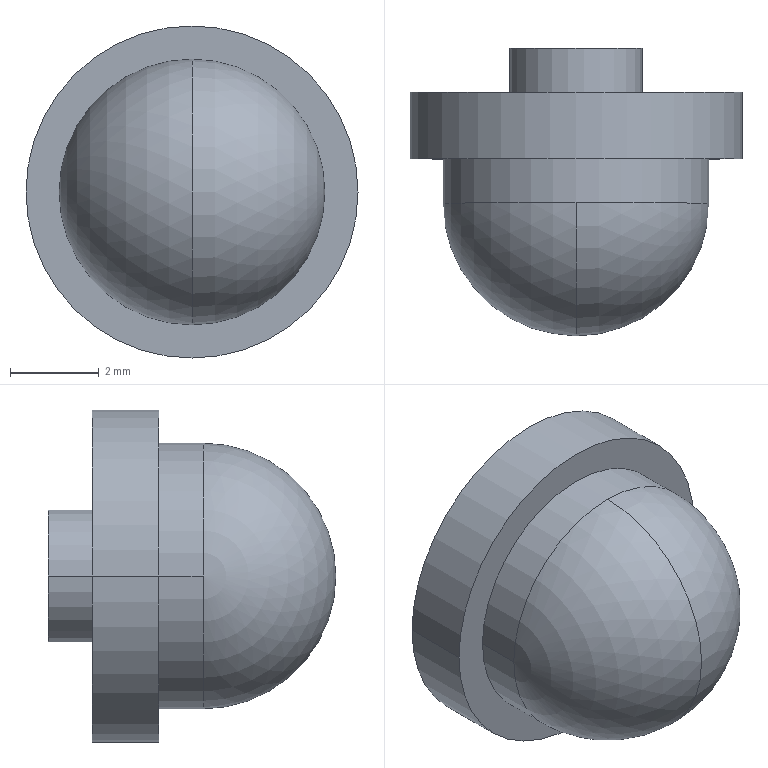Part | STEP file | SHS15C block-Part-2-7 | 1 solid | 11 faces | box 7.5 x 6.5 x 7.5 mm | volume 158.16 mm3 | cylinder 6 | plane 3 | sphere 2 | commonest cylinder face diameters 3 x2 6 x2 7.5 x2
STEP:
#1=CARTESIAN_POINT('',(0.,0.,0.));
#2=DIRECTION('',(0.,0.,1.));
#3=DIRECTION('',(1.,0.,0.));
#4=AXIS2_PLACEMENT_3D('',#1,#2,#3);
#5=CARTESIAN_POINT('',(61.7,-39.2,4.));
#6=VERTEX_POINT('',#5);
#7=CARTESIAN_POINT('',(58.7,-39.2,4.));
#8=VERTEX_POINT('',#7);
#9=CARTESIAN_POINT('',(60.2,-39.2,4.));
#10=DIRECTION('',(0.,-1.,0.));
#11=DIRECTION('',(-1.,0.,0.));
#12=AXIS2_PLACEMENT_3D('',#9,#10,#11);
#13=CIRCLE('',#12,1.5);
#14=CARTESIAN_POINT('',(60.2,-39.2,4.));
#15=DIRECTION('',(0.,-1.,0.));
#16=DIRECTION('',(1.,0.,0.));
#17=AXIS2_PLACEMENT_3D('',#14,#15,#16);
#18=CYLINDRICAL_SURFACE('',#17,1.5);
#19=CARTESIAN_POINT('',(-3.142,0.));
#20=DIRECTION('',(1.,0.));
#21=VECTOR('',#20,1.);
#22=LINE('',#19,#21);
#23=(GEOMETRIC_REPRESENTATION_CONTEXT(2)PARAMETRIC_REPRESENTATION_CONTEXT()REPRESENTATION_CONTEXT('',''));
#24=DEFINITIONAL_REPRESENTATION('',(#22),#23);
#25=PCURVE('',#18,#24);
#26=CARTESIAN_POINT('',(60.2,-39.2,4.));
#27=DIRECTION('',(0.,1.,0.));
#28=DIRECTION('',(-1.,0.,0.));
#29=AXIS2_PLACEMENT_3D('',#26,#27,#28);
#30=PLANE('',#29);
#31=CARTESIAN_POINT('',(1.5,0.));
#32=CARTESIAN_POINT('',(1.5,-2.598));
#33=CARTESIAN_POINT('',(-0.75,-1.299));
#34=CARTESIAN_POINT('',(-3.,0.));
#35=CARTESIAN_POINT('',(-0.75,1.299));
#36=CARTESIAN_POINT('',(1.5,2.598));
#37=CARTESIAN_POINT('',(1.5,0.));
#38=(BOUNDED_CURVE()B_SPLINE_CURVE(2,(#31,#32,#33,#34,#35,#36,#37),.UNSPECIFIED.,.T.,.F.)B_SPLINE_CURVE_WITH_KNOTS((1,2,2,2,2,1),(-2.094,0.,2.094,4.189,6.283,8.378),.UNSPECIFIED.)CURVE()GEOMETRIC_REPRESENTATION_ITEM()RATIONAL_B_SPLINE_CURVE((1.,0.5,1.,0.5,1.,0.5,1.))REPRESENTATION_ITEM(''));
#39=(GEOMETRIC_REPRESENTATION_CONTEXT(2)PARAMETRIC_REPRESENTATION_CONTEXT()REPRESENTATION_CONTEXT('',''));
#40=DEFINITIONAL_REPRESENTATION('',(#38),#39);
#41=PCURVE('',#30,#40);
#42=SURFACE_CURVE('',#13,(#25,#41),.PCURVE_S1.);
#43=EDGE_CURVE('',#6,#8,#42,.T.);
#44=ORIENTED_EDGE('',*,*,#43,.T.);
#45=CARTESIAN_POINT('',(58.7,-40.2,4.));
#46=VERTEX_POINT('',#45);
#47=CARTESIAN_POINT('',(58.7,-39.2,4.));
#48=DIRECTION('',(0.,-1.,0.));
#49=VECTOR('',#48,1.);
#50=LINE('',#47,#49);
#51=CARTESIAN_POINT('',(3.142,0.));
#52=DIRECTION('',(0.,1.));
#53=VECTOR('',#52,1.);
#54=LINE('',#51,#53);
#55=(GEOMETRIC_REPRESENTATION_CONTEXT(2)PARAMETRIC_REPRESENTATION_CONTEXT()REPRESENTATION_CONTEXT('',''));
#56=DEFINITIONAL_REPRESENTATION('',(#54),#55);
#57=PCURVE('',#18,#56);
#58=CARTESIAN_POINT('',(60.2,-39.2,4.));
#59=DIRECTION('',(0.,-1.,0.));
#60=DIRECTION('',(1.,0.,0.));
#61=AXIS2_PLACEMENT_3D('',#58,#59,#60);
#62=CYLINDRICAL_SURFACE('',#61,1.5);
#63=CARTESIAN_POINT('',(3.142,0.));
#64=DIRECTION('',(0.,1.));
#65=VECTOR('',#64,1.);
#66=LINE('',#63,#65);
#67=(GEOMETRIC_REPRESENTATION_CONTEXT(2)PARAMETRIC_REPRESENTATION_CONTEXT()REPRESENTATION_CONTEXT('',''));
#68=DEFINITIONAL_REPRESENTATION('',(#66),#67);
#69=PCURVE('',#62,#68);
#70=SURFACE_CURVE('',#50,(#57,#69),.PCURVE_S1.);
#71=EDGE_CURVE('',#8,#46,#70,.T.);
#72=ORIENTED_EDGE('',*,*,#71,.T.);
#73=CARTESIAN_POINT('',(61.7,-40.2,4.));
#74=VERTEX_POINT('',#73);
#75=CARTESIAN_POINT('',(60.2,-40.2,4.));
#76=DIRECTION('',(0.,-1.,0.));
#77=DIRECTION('',(-1.,0.,0.));
#78=AXIS2_PLACEMENT_3D('',#75,#76,#77);
#79=CIRCLE('',#78,1.5);
#80=CARTESIAN_POINT('',(-3.142,1.));
#81=DIRECTION('',(1.,0.));
#82=VECTOR('',#81,1.);
#83=LINE('',#80,#82);
#84=(GEOMETRIC_REPRESENTATION_CONTEXT(2)PARAMETRIC_REPRESENTATION_CONTEXT()REPRESENTATION_CONTEXT('',''));
#85=DEFINITIONAL_REPRESENTATION('',(#83),#84);
#86=PCURVE('',#18,#85);
#87=CARTESIAN_POINT('',(60.2,-40.2,0.25));
#88=DIRECTION('',(0.,-1.,0.));
#89=DIRECTION('',(1.,0.,0.));
#90=AXIS2_PLACEMENT_3D('',#87,#88,#89);
#91=PLANE('',#90);
#92=CARTESIAN_POINT('',(0.,3.75));
#93=DIRECTION('',(-1.,0.));
#94=AXIS2_PLACEMENT_2D('',#92,#93);
#95=CIRCLE('',#94,1.5);
#96=(GEOMETRIC_REPRESENTATION_CONTEXT(2)PARAMETRIC_REPRESENTATION_CONTEXT()REPRESENTATION_CONTEXT('',''));
#97=DEFINITIONAL_REPRESENTATION('',(#95),#96);
#98=PCURVE('',#91,#97);
#99=SURFACE_CURVE('',#79,(#86,#98),.PCURVE_S1.);
#100=EDGE_CURVE('',#74,#46,#99,.T.);
#101=ORIENTED_EDGE('',*,*,#100,.F.);
#102=CARTESIAN_POINT('',(61.7,-39.2,4.));
#103=DIRECTION('',(0.,-1.,0.));
#104=VECTOR('',#103,1.);
#105=LINE('',#102,#104);
#106=CARTESIAN_POINT('',(0.,0.));
#107=DIRECTION('',(0.,1.));
#108=VECTOR('',#107,1.);
#109=LINE('',#106,#108);
#110=(GEOMETRIC_REPRESENTATION_CONTEXT(2)PARAMETRIC_REPRESENTATION_CONTEXT()REPRESENTATION_CONTEXT('',''));
#111=DEFINITIONAL_REPRESENTATION('',(#109),#110);
#112=PCURVE('',#18,#111);
#113=CARTESIAN_POINT('',(6.283,0.));
#114=DIRECTION('',(0.,1.));
#115=VECTOR('',#114,1.);
#116=LINE('',#113,#115);
#117=(GEOMETRIC_REPRESENTATION_CONTEXT(2)PARAMETRIC_REPRESENTATION_CONTEXT()REPRESENTATION_CONTEXT('',''));
#118=DEFINITIONAL_REPRESENTATION('',(#116),#117);
#119=PCURVE('',#62,#118);
#120=SURFACE_CURVE('',#105,(#112,#119),.PCURVE_S1.);
#121=EDGE_CURVE('',#6,#74,#120,.T.);
#122=ORIENTED_EDGE('',*,*,#121,.F.);
#123=EDGE_LOOP('',(#44,#72,#101,#122));
#124=FACE_BOUND('',#123,.T.);
#125=ADVANCED_FACE('',(#124),#18,.T.);
#126=CARTESIAN_POINT('',(63.95,-41.7,4.));
#127=VERTEX_POINT('',#126);
#128=CARTESIAN_POINT('',(56.45,-41.7,4.));
#129=VERTEX_POINT('',#128);
#130=CARTESIAN_POINT('',(60.2,-41.7,4.));
#131=DIRECTION('',(0.,-1.,0.));
#132=DIRECTION('',(-1.,0.,0.));
#133=AXIS2_PLACEMENT_3D('',#130,#131,#132);
#134=CIRCLE('',#133,3.75);
#135=CARTESIAN_POINT('',(60.2,-35.7,4.));
#136=DIRECTION('',(0.,1.,0.));
#137=DIRECTION('',(-1.,0.,0.));
#138=AXIS2_PLACEMENT_3D('',#135,#136,#137);
#139=CYLINDRICAL_SURFACE('',#138,3.75);
#140=CARTESIAN_POINT('',(6.283,-6.));
#141=DIRECTION('',(-1.,0.));
#142=VECTOR('',#141,1.);
#143=LINE('',#140,#142);
#144=(GEOMETRIC_REPRESENTATION_CONTEXT(2)PARAMETRIC_REPRESENTATION_CONTEXT()REPRESENTATION_CONTEXT('',''));
#145=DEFINITIONAL_REPRESENTATION('',(#143),#144);
#146=PCURVE('',#139,#145);
#147=CARTESIAN_POINT('',(60.2,-41.7,1.));
#148=DIRECTION('',(0.,1.,0.));
#149=DIRECTION('',(-1.,0.,0.));
#150=AXIS2_PLACEMENT_3D('',#147,#148,#149);
#151=PLANE('',#150);
#152=CARTESIAN_POINT('',(3.75,3.));
#153=CARTESIAN_POINT('',(3.75,-3.495));
#154=CARTESIAN_POINT('',(-1.875,-0.2476));
#155=CARTESIAN_POINT('',(-7.5,3.));
#156=CARTESIAN_POINT('',(-1.875,6.248));
#157=CARTESIAN_POINT('',(3.75,9.495));
#158=CARTESIAN_POINT('',(3.75,3.));
#159=(BOUNDED_CURVE()B_SPLINE_CURVE(2,(#152,#153,#154,#155,#156,#157,#158),.UNSPECIFIED.,.T.,.F.)B_SPLINE_CURVE_WITH_KNOTS((1,2,2,2,2,1),(-2.094,0.,2.094,4.189,6.283,8.378),.UNSPECIFIED.)CURVE()GEOMETRIC_REPRESENTATION_ITEM()RATIONAL_B_SPLINE_CURVE((1.,0.5,1.,0.5,1.,0.5,1.))REPRESENTATION_ITEM(''));
#160=(GEOMETRIC_REPRESENTATION_CONTEXT(2)PARAMETRIC_REPRESENTATION_CONTEXT()REPRESENTATION_CONTEXT('',''));
#161=DEFINITIONAL_REPRESENTATION('',(#159),#160);
#162=PCURVE('',#151,#161);
#163=SURFACE_CURVE('',#134,(#146,#162),.PCURVE_S1.);
#164=EDGE_CURVE('',#127,#129,#163,.T.);
#165=ORIENTED_EDGE('',*,*,#164,.F.);
#166=CARTESIAN_POINT('',(63.95,-40.2,4.));
#167=VERTEX_POINT('',#166);
#168=CARTESIAN_POINT('',(63.95,-35.7,4.));
#169=DIRECTION('',(0.,1.,0.));
#170=VECTOR('',#169,1.);
#171=LINE('',#168,#170);
#172=CARTESIAN_POINT('',(3.142,0.));
#173=DIRECTION('',(0.,1.));
#174=VECTOR('',#173,1.);
#175=LINE('',#172,#174);
#176=(GEOMETRIC_REPRESENTATION_CONTEXT(2)PARAMETRIC_REPRESENTATION_CONTEXT()REPRESENTATION_CONTEXT('',''));
#177=DEFINITIONAL_REPRESENTATION('',(#175),#176);
#178=PCURVE('',#139,#177);
#179=CARTESIAN_POINT('',(60.2,-35.7,4.));
#180=DIRECTION('',(0.,1.,0.));
#181=DIRECTION('',(-1.,0.,0.));
#182=AXIS2_PLACEMENT_3D('',#179,#180,#181);
#183=CYLINDRICAL_SURFACE('',#182,3.75);
#184=CARTESIAN_POINT('',(3.142,0.));
#185=DIRECTION('',(0.,1.));
#186=VECTOR('',#185,1.);
#187=LINE('',#184,#186);
#188=(GEOMETRIC_REPRESENTATION_CONTEXT(2)PARAMETRIC_REPRESENTATION_CONTEXT()REPRESENTATION_CONTEXT('',''));
#189=DEFINITIONAL_REPRESENTATION('',(#187),#188);
#190=PCURVE('',#183,#189);
#191=SURFACE_CURVE('',#171,(#178,#190),.PCURVE_S1.);
#192=EDGE_CURVE('',#127,#167,#191,.T.);
#193=ORIENTED_EDGE('',*,*,#192,.T.);
#194=CARTESIAN_POINT('',(56.45,-40.2,4.));
#195=VERTEX_POINT('',#194);
#196=CARTESIAN_POINT('',(60.2,-40.2,4.));
#197=DIRECTION('',(0.,-1.,0.));
#198=DIRECTION('',(-1.,0.,0.));
#199=AXIS2_PLACEMENT_3D('',#196,#197,#198);
#200=CIRCLE('',#199,3.75);
#201=CARTESIAN_POINT('',(6.283,-4.5));
#202=DIRECTION('',(-1.,0.));
#203=VECTOR('',#202,1.);
#204=LINE('',#201,#203);
#205=(GEOMETRIC_REPRESENTATION_CONTEXT(2)PARAMETRIC_REPRESENTATION_CONTEXT()REPRESENTATION_CONTEXT('',''));
#206=DEFINITIONAL_REPRESENTATION('',(#204),#205);
#207=PCURVE('',#139,#206);
#208=CARTESIAN_POINT('',(0.,3.75));
#209=DIRECTION('',(-1.,0.));
#210=AXIS2_PLACEMENT_2D('',#208,#209);
#211=CIRCLE('',#210,3.75);
#212=(GEOMETRIC_REPRESENTATION_CONTEXT(2)PARAMETRIC_REPRESENTATION_CONTEXT()REPRESENTATION_CONTEXT('',''));
#213=DEFINITIONAL_REPRESENTATION('',(#211),#212);
#214=PCURVE('',#91,#213);
#215=SURFACE_CURVE('',#200,(#207,#214),.PCURVE_S1.);
#216=EDGE_CURVE('',#167,#195,#215,.T.);
#217=ORIENTED_EDGE('',*,*,#216,.T.);
#218=CARTESIAN_POINT('',(56.45,-35.7,4.));
#219=DIRECTION('',(0.,1.,0.));
#220=VECTOR('',#219,1.);
#221=LINE('',#218,#220);
#222=CARTESIAN_POINT('',(0.,0.));
#223=DIRECTION('',(0.,1.));
#224=VECTOR('',#223,1.);
#225=LINE('',#222,#224);
#226=(GEOMETRIC_REPRESENTATION_CONTEXT(2)PARAMETRIC_REPRESENTATION_CONTEXT()REPRESENTATION_CONTEXT('',''));
#227=DEFINITIONAL_REPRESENTATION('',(#225),#226);
#228=PCURVE('',#139,#227);
#229=CARTESIAN_POINT('',(6.283,0.));
#230=DIRECTION('',(0.,1.));
#231=VECTOR('',#230,1.);
#232=LINE('',#229,#231);
#233=(GEOMETRIC_REPRESENTATION_CONTEXT(2)PARAMETRIC_REPRESENTATION_CONTEXT()REPRESENTATION_CONTEXT('',''));
#234=DEFINITIONAL_REPRESENTATION('',(#232),#233);
#235=PCURVE('',#183,#234);
#236=SURFACE_CURVE('',#221,(#228,#235),.PCURVE_S1.);
#237=EDGE_CURVE('',#129,#195,#236,.T.);
#238=ORIENTED_EDGE('',*,*,#237,.F.);
#239=EDGE_LOOP('',(#165,#193,#217,#238));
#240=FACE_BOUND('',#239,.T.);
#241=ADVANCED_FACE('',(#240),#139,.T.);
#242=CARTESIAN_POINT('',(63.2,-42.7,4.));
#243=VERTEX_POINT('',#242);
#244=CARTESIAN_POINT('',(60.2,-42.7,7.));
#245=VERTEX_POINT('',#244);
#246=CARTESIAN_POINT('',(60.2,-42.7,4.));
#247=DIRECTION('',(0.,-1.,0.));
#248=DIRECTION('',(-1.,0.,0.));
#249=AXIS2_PLACEMENT_3D('',#246,#247,#248);
#250=CIRCLE('',#249,3.);
#251=CARTESIAN_POINT('',(60.2,-35.7,4.));
#252=DIRECTION('',(0.,1.,0.));
#253=DIRECTION('',(-1.,0.,0.));
#254=AXIS2_PLACEMENT_3D('',#251,#252,#253);
#255=CYLINDRICAL_SURFACE('',#254,3.);
#256=CARTESIAN_POINT('',(6.283,-7.));
#257=DIRECTION('',(-1.,0.));
#258=VECTOR('',#257,1.);
#259=LINE('',#256,#258);
#260=(GEOMETRIC_REPRESENTATION_CONTEXT(2)PARAMETRIC_REPRESENTATION_CONTEXT()REPRESENTATION_CONTEXT('',''));
#261=DEFINITIONAL_REPRESENTATION('',(#259),#260);
#262=PCURVE('',#255,#261);
#263=CARTESIAN_POINT('',(60.2,-42.7,4.));
#264=DIRECTION('',(-1.,0.,0.));
#265=DIRECTION('',(0.,0.,-1.));
#266=AXIS2_PLACEMENT_3D('',#263,#264,#265);
#267=SPHERICAL_SURFACE('',#266,3.);
#268=CARTESIAN_POINT('',(3.142,-1.571));
#269=CARTESIAN_POINT('',(3.142,-1.547));
#270=CARTESIAN_POINT('',(3.142,-1.499));
#271=CARTESIAN_POINT('',(3.142,-1.428));
#272=CARTESIAN_POINT('',(3.142,-1.357));
#273=CARTESIAN_POINT('',(3.142,-1.285));
#274=CARTESIAN_POINT('',(3.142,-1.214));
#275=CARTESIAN_POINT('',(3.142,-1.142));
#276=CARTESIAN_POINT('',(3.142,-1.071));
#277=CARTESIAN_POINT('',(3.142,-0.9996));
#278=CARTESIAN_POINT('',(3.142,-0.9282));
#279=CARTESIAN_POINT('',(3.142,-0.8568));
#280=CARTESIAN_POINT('',(3.142,-0.7854));
#281=CARTESIAN_POINT('',(3.142,-0.714));
#282=CARTESIAN_POINT('',(3.142,-0.6426));
#283=CARTESIAN_POINT('',(3.142,-0.5712));
#284=CARTESIAN_POINT('',(3.142,-0.4998));
#285=CARTESIAN_POINT('',(3.142,-0.4284));
#286=CARTESIAN_POINT('',(3.142,-0.357));
#287=CARTESIAN_POINT('',(3.142,-0.2856));
#288=CARTESIAN_POINT('',(3.142,-0.2142));
#289=CARTESIAN_POINT('',(3.142,-0.1428));
#290=CARTESIAN_POINT('',(3.142,-0.0714));
#291=CARTESIAN_POINT('',(3.142,-0.0238));
#292=CARTESIAN_POINT('',(3.142,0.));
#293=B_SPLINE_CURVE_WITH_KNOTS('',3,(#268,#269,#270,#271,#272,#273,#274,#275,#276,#277,#278,#279,#280,#281,#282,#283,#284,#285,#286,#287,#288,#289,#290,#291,#292),.UNSPECIFIED.,.F.,.F.,(4,1,1,1,1,1,1,1,1,1,1,1,1,1,1,1,1,1,1,1,1,1,4),(3.142,3.213,3.284,3.356,3.427,3.499,3.57,3.641,3.713,3.784,3.856,3.927,3.998,4.07,4.141,4.213,4.284,4.355,4.427,4.498,4.57,4.641,4.712),.QUASI_UNIFORM_KNOTS.);
#294=(GEOMETRIC_REPRESENTATION_CONTEXT(2)PARAMETRIC_REPRESENTATION_CONTEXT()REPRESENTATION_CONTEXT('',''));
#295=DEFINITIONAL_REPRESENTATION('',(#293),#294);
#296=PCURVE('',#267,#295);
#297=SURFACE_CURVE('',#250,(#262,#296),.PCURVE_S1.);
#298=EDGE_CURVE('',#243,#245,#297,.T.);
#299=ORIENTED_EDGE('',*,*,#298,.F.);
#300=CARTESIAN_POINT('',(63.2,-41.7,4.));
#301=VERTEX_POINT('',#300);
#302=CARTESIAN_POINT('',(63.2,-35.7,4.));
#303=DIRECTION('',(0.,1.,0.));
#304=VECTOR('',#303,1.);
#305=LINE('',#302,#304);
#306=CARTESIAN_POINT('',(3.142,0.));
#307=DIRECTION('',(0.,1.));
#308=VECTOR('',#307,1.);
#309=LINE('',#306,#308);
#310=(GEOMETRIC_REPRESENTATION_CONTEXT(2)PARAMETRIC_REPRESENTATION_CONTEXT()REPRESENTATION_CONTEXT('',''));
#311=DEFINITIONAL_REPRESENTATION('',(#309),#310);
#312=PCURVE('',#255,#311);
#313=CARTESIAN_POINT('',(60.2,-35.7,4.));
#314=DIRECTION('',(0.,1.,0.));
#315=DIRECTION('',(-1.,0.,0.));
#316=AXIS2_PLACEMENT_3D('',#313,#314,#315);
#317=CYLINDRICAL_SURFACE('',#316,3.);
#318=CARTESIAN_POINT('',(3.142,0.));
#319=DIRECTION('',(0.,1.));
#320=VECTOR('',#319,1.);
#321=LINE('',#318,#320);
#322=(GEOMETRIC_REPRESENTATION_CONTEXT(2)PARAMETRIC_REPRESENTATION_CONTEXT()REPRESENTATION_CONTEXT('',''));
#323=DEFINITIONAL_REPRESENTATION('',(#321),#322);
#324=PCURVE('',#317,#323);
#325=SURFACE_CURVE('',#305,(#312,#324),.PCURVE_S1.);
#326=EDGE_CURVE('',#243,#301,#325,.T.);
#327=ORIENTED_EDGE('',*,*,#326,.T.);
#328=CARTESIAN_POINT('',(57.2,-41.7,4.));
#329=VERTEX_POINT('',#328);
#330=CARTESIAN_POINT('',(60.2,-41.7,4.));
#331=DIRECTION('',(0.,-1.,0.));
#332=DIRECTION('',(-1.,0.,0.));
#333=AXIS2_PLACEMENT_3D('',#330,#331,#332);
#334=CIRCLE('',#333,3.);
#335=CARTESIAN_POINT('',(6.283,-6.));
#336=DIRECTION('',(-1.,0.));
#337=VECTOR('',#336,1.);
#338=LINE('',#335,#337);
#339=(GEOMETRIC_REPRESENTATION_CONTEXT(2)PARAMETRIC_REPRESENTATION_CONTEXT()REPRESENTATION_CONTEXT('',''));
#340=DEFINITIONAL_REPRESENTATION('',(#338),#339);
#341=PCURVE('',#255,#340);
#342=CARTESIAN_POINT('',(3.,3.));
#343=CARTESIAN_POINT('',(3.,-2.196));
#344=CARTESIAN_POINT('',(-1.5,0.4019));
#345=CARTESIAN_POINT('',(-6.,3.));
#346=CARTESIAN_POINT('',(-1.5,5.598));
#347=CARTESIAN_POINT('',(3.,8.196));
#348=CARTESIAN_POINT('',(3.,3.));
#349=(BOUNDED_CURVE()B_SPLINE_CURVE(2,(#342,#343,#344,#345,#346,#347,#348),.UNSPECIFIED.,.T.,.F.)B_SPLINE_CURVE_WITH_KNOTS((1,2,2,2,2,1),(-2.094,0.,2.094,4.189,6.283,8.378),.UNSPECIFIED.)CURVE()GEOMETRIC_REPRESENTATION_ITEM()RATIONAL_B_SPLINE_CURVE((1.,0.5,1.,0.5,1.,0.5,1.))REPRESENTATION_ITEM(''));
#350=(GEOMETRIC_REPRESENTATION_CONTEXT(2)PARAMETRIC_REPRESENTATION_CONTEXT()REPRESENTATION_CONTEXT('',''));
#351=DEFINITIONAL_REPRESENTATION('',(#349),#350);
#352=PCURVE('',#151,#351);
#353=SURFACE_CURVE('',#334,(#341,#352),.PCURVE_S1.);
#354=EDGE_CURVE('',#301,#329,#353,.T.);
#355=ORIENTED_EDGE('',*,*,#354,.T.);
#356=CARTESIAN_POINT('',(57.2,-42.7,4.));
#357=VERTEX_POINT('',#356);
#358=CARTESIAN_POINT('',(57.2,-35.7,4.));
#359=DIRECTION('',(0.,1.,0.));
#360=VECTOR('',#359,1.);
#361=LINE('',#358,#360);
#362=CARTESIAN_POINT('',(0.,0.));
#363=DIRECTION('',(0.,1.));
#364=VECTOR('',#363,1.);
#365=LINE('',#362,#364);
#366=(GEOMETRIC_REPRESENTATION_CONTEXT(2)PARAMETRIC_REPRESENTATION_CONTEXT()REPRESENTATION_CONTEXT('',''));
#367=DEFINITIONAL_REPRESENTATION('',(#365),#366);
#368=PCURVE('',#255,#367);
#369=CARTESIAN_POINT('',(6.283,0.));
#370=DIRECTION('',(0.,1.));
#371=VECTOR('',#370,1.);
#372=LINE('',#369,#371);
#373=(GEOMETRIC_REPRESENTATION_CONTEXT(2)PARAMETRIC_REPRESENTATION_CONTEXT()REPRESENTATION_CONTEXT('',''));
#374=DEFINITIONAL_REPRESENTATION('',(#372),#373);
#375=PCURVE('',#317,#374);
#376=SURFACE_CURVE('',#361,(#368,#375),.PCURVE_S1.);
#377=EDGE_CURVE('',#357,#329,#376,.T.);
#378=ORIENTED_EDGE('',*,*,#377,.F.);
#379=CARTESIAN_POINT('',(60.2,-42.7,4.));
#380=DIRECTION('',(0.,-1.,0.));
#381=DIRECTION('',(-1.,0.,0.));
#382=AXIS2_PLACEMENT_3D('',#379,#380,#381);
#383=CIRCLE('',#382,3.);
#384=CARTESIAN_POINT('',(6.283,-7.));
#385=DIRECTION('',(-1.,0.));
#386=VECTOR('',#385,1.);
#387=LINE('',#384,#386);
#388=(GEOMETRIC_REPRESENTATION_CONTEXT(2)PARAMETRIC_REPRESENTATION_CONTEXT()REPRESENTATION_CONTEXT('',''));
#389=DEFINITIONAL_REPRESENTATION('',(#387),#388);
#390=PCURVE('',#255,#389);
#391=CARTESIAN_POINT('',(60.2,-42.7,4.));
#392=DIRECTION('',(-1.,0.,0.));
#393=DIRECTION('',(0.,0.,-1.));
#394=AXIS2_PLACEMENT_3D('',#391,#392,#393);
#395=SPHERICAL_SURFACE('',#394,3.);
#396=CARTESIAN_POINT('',(3.142,-4.712));
#397=DIRECTION('',(0.,1.));
#398=VECTOR('',#397,1.);
#399=LINE('',#396,#398);
#400=(GEOMETRIC_REPRESENTATION_CONTEXT(2)PARAMETRIC_REPRESENTATION_CONTEXT()REPRESENTATION_CONTEXT('',''));
#401=DEFINITIONAL_REPRESENTATION('',(#399),#400);
#402=PCURVE('',#395,#401);
#403=SURFACE_CURVE('',#383,(#390,#402),.PCURVE_S1.);
#404=EDGE_CURVE('',#245,#357,#403,.T.);
#405=ORIENTED_EDGE('',*,*,#404,.F.);
#406=EDGE_LOOP('',(#299,#327,#355,#378,#405));
#407=FACE_BOUND('',#406,.T.);
#408=ADVANCED_FACE('',(#407),#255,.T.);
#409=CARTESIAN_POINT('',(60.2,-45.7,4.));
#410=VERTEX_POINT('',#409);
#411=CARTESIAN_POINT('',(60.2,-42.7,1.));
#412=VERTEX_POINT('',#411);
#413=CARTESIAN_POINT('',(60.2,-42.7,4.));
#414=DIRECTION('',(1.,0.,0.));
#415=DIRECTION('',(0.,0.,-1.));
#416=AXIS2_PLACEMENT_3D('',#413,#414,#415);
#417=CIRCLE('',#416,3.);
#418=CARTESIAN_POINT('',(6.283,0.));
#419=DIRECTION('',(-1.,0.));
#420=VECTOR('',#419,1.);
#421=LINE('',#418,#420);
#422=(GEOMETRIC_REPRESENTATION_CONTEXT(2)PARAMETRIC_REPRESENTATION_CONTEXT()REPRESENTATION_CONTEXT('',''));
#423=DEFINITIONAL_REPRESENTATION('',(#421),#422);
#424=PCURVE('',#395,#423);
#425=CARTESIAN_POINT('',(6.283,0.));
#426=DIRECTION('',(-1.,0.));
#427=VECTOR('',#426,1.);
#428=LINE('',#425,#427);
#429=(GEOMETRIC_REPRESENTATION_CONTEXT(2)PARAMETRIC_REPRESENTATION_CONTEXT()REPRESENTATION_CONTEXT('',''));
#430=DEFINITIONAL_REPRESENTATION('',(#428),#429);
#431=PCURVE('',#267,#430);
#432=SURFACE_CURVE('',#417,(#424,#431),.PCURVE_S1.);
#433=EDGE_CURVE('',#410,#412,#432,.T.);
#434=ORIENTED_EDGE('',*,*,#433,.F.);
#435=CARTESIAN_POINT('',(60.2,-42.7,4.));
#436=DIRECTION('',(-1.,0.,0.));
#437=DIRECTION('',(0.,0.,1.));
#438=AXIS2_PLACEMENT_3D('',#435,#436,#437);
#439=CIRCLE('',#438,3.);
#440=CARTESIAN_POINT('',(-3.142,0.));
#441=DIRECTION('',(1.,0.));
#442=VECTOR('',#441,1.);
#443=LINE('',#440,#442);
#444=(GEOMETRIC_REPRESENTATION_CONTEXT(2)PARAMETRIC_REPRESENTATION_CONTEXT()REPRESENTATION_CONTEXT('',''));
#445=DEFINITIONAL_REPRESENTATION('',(#443),#444);
#446=PCURVE('',#395,#445);
#447=CARTESIAN_POINT('',(-3.142,0.));
#448=DIRECTION('',(1.,0.));
#449=VECTOR('',#448,1.);
#450=LINE('',#447,#449);
#451=(GEOMETRIC_REPRESENTATION_CONTEXT(2)PARAMETRIC_REPRESENTATION_CONTEXT()REPRESENTATION_CONTEXT('',''));
#452=DEFINITIONAL_REPRESENTATION('',(#450),#451);
#453=PCURVE('',#267,#452);
#454=SURFACE_CURVE('',#439,(#446,#453),.PCURVE_S1.);
#455=EDGE_CURVE('',#410,#245,#454,.T.);
#456=ORIENTED_EDGE('',*,*,#455,.T.);
#457=ORIENTED_EDGE('',*,*,#404,.T.);
#458=CARTESIAN_POINT('',(60.2,-42.7,4.));
#459=DIRECTION('',(0.,-1.,0.));
#460=DIRECTION('',(-1.,0.,0.));
#461=AXIS2_PLACEMENT_3D('',#458,#459,#460);
#462=CIRCLE('',#461,3.);
#463=CARTESIAN_POINT('',(0.,1.571));
#464=DIRECTION('',(0.,-1.));
#465=VECTOR('',#464,1.);
#466=LINE('',#463,#465);
#467=(GEOMETRIC_REPRESENTATION_CONTEXT(2)PARAMETRIC_REPRESENTATION_CONTEXT()REPRESENTATION_CONTEXT('',''));
#468=DEFINITIONAL_REPRESENTATION('',(#466),#467);
#469=PCURVE('',#395,#468);
#470=CARTESIAN_POINT('',(6.283,-7.));
#471=DIRECTION('',(-1.,0.));
#472=VECTOR('',#471,1.);
#473=LINE('',#470,#472);
#474=(GEOMETRIC_REPRESENTATION_CONTEXT(2)PARAMETRIC_REPRESENTATION_CONTEXT()REPRESENTATION_CONTEXT('',''));
#475=DEFINITIONAL_REPRESENTATION('',(#473),#474);
#476=PCURVE('',#317,#475);
#477=SURFACE_CURVE('',#462,(#469,#476),.PCURVE_S1.);
#478=EDGE_CURVE('',#357,#412,#477,.T.);
#479=ORIENTED_EDGE('',*,*,#478,.T.);
#480=EDGE_LOOP('',(#434,#456,#457,#479));
#481=FACE_BOUND('',#480,.T.);
#482=ADVANCED_FACE('',(#481),#395,.T.);
#483=ORIENTED_EDGE('',*,*,#455,.F.);
#484=ORIENTED_EDGE('',*,*,#433,.T.);
#485=CARTESIAN_POINT('',(60.2,-42.7,4.));
#486=DIRECTION('',(0.,-1.,0.));
#487=DIRECTION('',(-1.,0.,0.));
#488=AXIS2_PLACEMENT_3D('',#485,#486,#487);
#489=CIRCLE('',#488,3.);
#490=CARTESIAN_POINT('',(0.,1.571));
#491=DIRECTION('',(0.,-1.));
#492=VECTOR('',#491,1.);
#493=LINE('',#490,#492);
#494=(GEOMETRIC_REPRESENTATION_CONTEXT(2)PARAMETRIC_REPRESENTATION_CONTEXT()REPRESENTATION_CONTEXT('',''));
#495=DEFINITIONAL_REPRESENTATION('',(#493),#494);
#496=PCURVE('',#267,#495);
#497=CARTESIAN_POINT('',(6.283,-7.));
#498=DIRECTION('',(-1.,0.));
#499=VECTOR('',#498,1.);
#500=LINE('',#497,#499);
#501=(GEOMETRIC_REPRESENTATION_CONTEXT(2)PARAMETRIC_REPRESENTATION_CONTEXT()REPRESENTATION_CONTEXT('',''));
#502=DEFINITIONAL_REPRESENTATION('',(#500),#501);
#503=PCURVE('',#317,#502);
#504=SURFACE_CURVE('',#489,(#496,#503),.PCURVE_S1.);
#505=EDGE_CURVE('',#412,#243,#504,.T.);
#506=ORIENTED_EDGE('',*,*,#505,.T.);
#507=ORIENTED_EDGE('',*,*,#298,.T.);
#508=EDGE_LOOP('',(#483,#484,#506,#507));
#509=FACE_BOUND('',#508,.T.);
#510=ADVANCED_FACE('',(#509),#267,.T.);
#511=ORIENTED_EDGE('',*,*,#326,.F.);
#512=ORIENTED_EDGE('',*,*,#505,.F.);
#513=ORIENTED_EDGE('',*,*,#478,.F.);
#514=ORIENTED_EDGE('',*,*,#377,.T.);
#515=CARTESIAN_POINT('',(60.2,-41.7,4.));
#516=DIRECTION('',(0.,-1.,0.));
#517=DIRECTION('',(-1.,0.,0.));
#518=AXIS2_PLACEMENT_3D('',#515,#516,#517);
#519=CIRCLE('',#518,3.);
#520=CARTESIAN_POINT('',(6.283,-6.));
#521=DIRECTION('',(-1.,0.));
#522=VECTOR('',#521,1.);
#523=LINE('',#520,#522);
#524=(GEOMETRIC_REPRESENTATION_CONTEXT(2)PARAMETRIC_REPRESENTATION_CONTEXT()REPRESENTATION_CONTEXT('',''));
#525=DEFINITIONAL_REPRESENTATION('',(#523),#524);
#526=PCURVE('',#317,#525);
#527=CARTESIAN_POINT('',(3.,3.));
#528=CARTESIAN_POINT('',(3.,-2.196));
#529=CARTESIAN_POINT('',(-1.5,0.4019));
#530=CARTESIAN_POINT('',(-6.,3.));
#531=CARTESIAN_POINT('',(-1.5,5.598));
#532=CARTESIAN_POINT('',(3.,8.196));
#533=CARTESIAN_POINT('',(3.,3.));
#534=(BOUNDED_CURVE()B_SPLINE_CURVE(2,(#527,#528,#529,#530,#531,#532,#533),.UNSPECIFIED.,.T.,.F.)B_SPLINE_CURVE_WITH_KNOTS((1,2,2,2,2,1),(-2.094,0.,2.094,4.189,6.283,8.378),.UNSPECIFIED.)CURVE()GEOMETRIC_REPRESENTATION_ITEM()RATIONAL_B_SPLINE_CURVE((1.,0.5,1.,0.5,1.,0.5,1.))REPRESENTATION_ITEM(''));
#535=(GEOMETRIC_REPRESENTATION_CONTEXT(2)PARAMETRIC_REPRESENTATION_CONTEXT()REPRESENTATION_CONTEXT('',''));
#536=DEFINITIONAL_REPRESENTATION('',(#534),#535);
#537=PCURVE('',#151,#536);
#538=SURFACE_CURVE('',#519,(#526,#537),.PCURVE_S1.);
#539=EDGE_CURVE('',#329,#301,#538,.T.);
#540=ORIENTED_EDGE('',*,*,#539,.T.);
#541=EDGE_LOOP('',(#511,#512,#513,#514,#540));
#542=FACE_BOUND('',#541,.T.);
#543=ADVANCED_FACE('',(#542),#317,.T.);
#544=CARTESIAN_POINT('',(60.2,-41.7,4.));
#545=DIRECTION('',(0.,-1.,0.));
#546=DIRECTION('',(-1.,0.,0.));
#547=AXIS2_PLACEMENT_3D('',#544,#545,#546);
#548=CIRCLE('',#547,3.75);
#549=CARTESIAN_POINT('',(3.75,3.));
#550=CARTESIAN_POINT('',(3.75,-3.495));
#551=CARTESIAN_POINT('',(-1.875,-0.2476));
#552=CARTESIAN_POINT('',(-7.5,3.));
#553=CARTESIAN_POINT('',(-1.875,6.248));
#554=CARTESIAN_POINT('',(3.75,9.495));
#555=CARTESIAN_POINT('',(3.75,3.));
#556=(BOUNDED_CURVE()B_SPLINE_CURVE(2,(#549,#550,#551,#552,#553,#554,#555),.UNSPECIFIED.,.T.,.F.)B_SPLINE_CURVE_WITH_KNOTS((1,2,2,2,2,1),(-2.094,0.,2.094,4.189,6.283,8.378),.UNSPECIFIED.)CURVE()GEOMETRIC_REPRESENTATION_ITEM()RATIONAL_B_SPLINE_CURVE((1.,0.5,1.,0.5,1.,0.5,1.))REPRESENTATION_ITEM(''));
#557=(GEOMETRIC_REPRESENTATION_CONTEXT(2)PARAMETRIC_REPRESENTATION_CONTEXT()REPRESENTATION_CONTEXT('',''));
#558=DEFINITIONAL_REPRESENTATION('',(#556),#557);
#559=PCURVE('',#151,#558);
#560=CARTESIAN_POINT('',(6.283,-6.));
#561=DIRECTION('',(-1.,0.));
#562=VECTOR('',#561,1.);
#563=LINE('',#560,#562);
#564=(GEOMETRIC_REPRESENTATION_CONTEXT(2)PARAMETRIC_REPRESENTATION_CONTEXT()REPRESENTATION_CONTEXT('',''));
#565=DEFINITIONAL_REPRESENTATION('',(#563),#564);
#566=PCURVE('',#183,#565);
#567=SURFACE_CURVE('',#548,(#559,#566),.PCURVE_S1.);
#568=EDGE_CURVE('',#129,#127,#567,.T.);
#569=ORIENTED_EDGE('',*,*,#568,.T.);
#570=ORIENTED_EDGE('',*,*,#164,.T.);
#571=EDGE_LOOP('',(#569,#570));
#572=FACE_BOUND('',#571,.T.);
#573=ORIENTED_EDGE('',*,*,#539,.F.);
#574=ORIENTED_EDGE('',*,*,#354,.F.);
#575=EDGE_LOOP('',(#573,#574));
#576=FACE_BOUND('',#575,.T.);
#577=ADVANCED_FACE('',(#572,#576),#151,.F.);
#578=ORIENTED_EDGE('',*,*,#192,.F.);
#579=ORIENTED_EDGE('',*,*,#568,.F.);
#580=ORIENTED_EDGE('',*,*,#237,.T.);
#581=CARTESIAN_POINT('',(60.2,-40.2,4.));
#582=DIRECTION('',(0.,-1.,0.));
#583=DIRECTION('',(-1.,0.,0.));
#584=AXIS2_PLACEMENT_3D('',#581,#582,#583);
#585=CIRCLE('',#584,3.75);
#586=CARTESIAN_POINT('',(6.283,-4.5));
#587=DIRECTION('',(-1.,0.));
#588=VECTOR('',#587,1.);
#589=LINE('',#586,#588);
#590=(GEOMETRIC_REPRESENTATION_CONTEXT(2)PARAMETRIC_REPRESENTATION_CONTEXT()REPRESENTATION_CONTEXT('',''));
#591=DEFINITIONAL_REPRESENTATION('',(#589),#590);
#592=PCURVE('',#183,#591);
#593=CARTESIAN_POINT('',(0.,3.75));
#594=DIRECTION('',(-1.,0.));
#595=AXIS2_PLACEMENT_2D('',#593,#594);
#596=CIRCLE('',#595,3.75);
#597=(GEOMETRIC_REPRESENTATION_CONTEXT(2)PARAMETRIC_REPRESENTATION_CONTEXT()REPRESENTATION_CONTEXT('',''));
#598=DEFINITIONAL_REPRESENTATION('',(#596),#597);
#599=PCURVE('',#91,#598);
#600=SURFACE_CURVE('',#585,(#592,#599),.PCURVE_S1.);
#601=EDGE_CURVE('',#195,#167,#600,.T.);
#602=ORIENTED_EDGE('',*,*,#601,.T.);
#603=EDGE_LOOP('',(#578,#579,#580,#602));
#604=FACE_BOUND('',#603,.T.);
#605=ADVANCED_FACE('',(#604),#183,.T.);
#606=ORIENTED_EDGE('',*,*,#601,.F.);
#607=ORIENTED_EDGE('',*,*,#216,.F.);
#608=EDGE_LOOP('',(#606,#607));
#609=FACE_BOUND('',#608,.T.);
#610=ORIENTED_EDGE('',*,*,#100,.T.);
#611=CARTESIAN_POINT('',(60.2,-40.2,4.));
#612=DIRECTION('',(0.,-1.,0.));
#613=DIRECTION('',(-1.,0.,0.));
#614=AXIS2_PLACEMENT_3D('',#611,#612,#613);
#615=CIRCLE('',#614,1.5);
#616=CARTESIAN_POINT('',(0.,3.75));
#617=DIRECTION('',(-1.,0.));
#618=AXIS2_PLACEMENT_2D('',#616,#617);
#619=CIRCLE('',#618,1.5);
#620=(GEOMETRIC_REPRESENTATION_CONTEXT(2)PARAMETRIC_REPRESENTATION_CONTEXT()REPRESENTATION_CONTEXT('',''));
#621=DEFINITIONAL_REPRESENTATION('',(#619),#620);
#622=PCURVE('',#91,#621);
#623=CARTESIAN_POINT('',(3.142,1.));
#624=DIRECTION('',(1.,0.));
#625=VECTOR('',#624,1.);
#626=LINE('',#623,#625);
#627=(GEOMETRIC_REPRESENTATION_CONTEXT(2)PARAMETRIC_REPRESENTATION_CONTEXT()REPRESENTATION_CONTEXT('',''));
#628=DEFINITIONAL_REPRESENTATION('',(#626),#627);
#629=PCURVE('',#62,#628);
#630=SURFACE_CURVE('',#615,(#622,#629),.PCURVE_S1.);
#631=EDGE_CURVE('',#46,#74,#630,.T.);
#632=ORIENTED_EDGE('',*,*,#631,.T.);
#633=EDGE_LOOP('',(#610,#632));
#634=FACE_BOUND('',#633,.T.);
#635=ADVANCED_FACE('',(#609,#634),#91,.F.);
#636=ORIENTED_EDGE('',*,*,#71,.F.);
#637=CARTESIAN_POINT('',(60.2,-39.2,4.));
#638=DIRECTION('',(0.,-1.,0.));
#639=DIRECTION('',(-1.,0.,0.));
#640=AXIS2_PLACEMENT_3D('',#637,#638,#639);
#641=CIRCLE('',#640,1.5);
#642=CARTESIAN_POINT('',(3.142,0.));
#643=DIRECTION('',(1.,0.));
#644=VECTOR('',#643,1.);
#645=LINE('',#642,#644);
#646=(GEOMETRIC_REPRESENTATION_CONTEXT(2)PARAMETRIC_REPRESENTATION_CONTEXT()REPRESENTATION_CONTEXT('',''));
#647=DEFINITIONAL_REPRESENTATION('',(#645),#646);
#648=PCURVE('',#62,#647);
#649=CARTESIAN_POINT('',(1.5,0.));
#650=CARTESIAN_POINT('',(1.5,-2.598));
#651=CARTESIAN_POINT('',(-0.75,-1.299));
#652=CARTESIAN_POINT('',(-3.,0.));
#653=CARTESIAN_POINT('',(-0.75,1.299));
#654=CARTESIAN_POINT('',(1.5,2.598));
#655=CARTESIAN_POINT('',(1.5,0.));
#656=(BOUNDED_CURVE()B_SPLINE_CURVE(2,(#649,#650,#651,#652,#653,#654,#655),.UNSPECIFIED.,.T.,.F.)B_SPLINE_CURVE_WITH_KNOTS((1,2,2,2,2,1),(-2.094,0.,2.094,4.189,6.283,8.378),.UNSPECIFIED.)CURVE()GEOMETRIC_REPRESENTATION_ITEM()RATIONAL_B_SPLINE_CURVE((1.,0.5,1.,0.5,1.,0.5,1.))REPRESENTATION_ITEM(''));
#657=(GEOMETRIC_REPRESENTATION_CONTEXT(2)PARAMETRIC_REPRESENTATION_CONTEXT()REPRESENTATION_CONTEXT('',''));
#658=DEFINITIONAL_REPRESENTATION('',(#656),#657);
#659=PCURVE('',#30,#658);
#660=SURFACE_CURVE('',#641,(#648,#659),.PCURVE_S1.);
#661=EDGE_CURVE('',#8,#6,#660,.T.);
#662=ORIENTED_EDGE('',*,*,#661,.T.);
#663=ORIENTED_EDGE('',*,*,#121,.T.);
#664=ORIENTED_EDGE('',*,*,#631,.F.);
#665=EDGE_LOOP('',(#636,#662,#663,#664));
#666=FACE_BOUND('',#665,.T.);
#667=ADVANCED_FACE('',(#666),#62,.T.);
#668=ORIENTED_EDGE('',*,*,#43,.F.);
#669=ORIENTED_EDGE('',*,*,#661,.F.);
#670=EDGE_LOOP('',(#668,#669));
#671=FACE_BOUND('',#670,.T.);
#672=ADVANCED_FACE('',(#671),#30,.T.);
#673=CLOSED_SHELL('',(#125,#241,#408,#482,#510,#543,#577,#605,#635,#667,#672));
#674=MANIFOLD_SOLID_BREP('',#673);
#675=(LENGTH_UNIT()NAMED_UNIT(*)SI_UNIT(.MILLI.,.METRE.));
#676=UNCERTAINTY_MEASURE_WITH_UNIT(LENGTH_MEASURE(0.0000001),#675,'','');
#677=(NAMED_UNIT(*)PLANE_ANGLE_UNIT()SI_UNIT($,.RADIAN.));
#678=(NAMED_UNIT(*)SI_UNIT($,.STERADIAN.)SOLID_ANGLE_UNIT());
#679=(GEOMETRIC_REPRESENTATION_CONTEXT(3)GLOBAL_UNCERTAINTY_ASSIGNED_CONTEXT((#676))GLOBAL_UNIT_ASSIGNED_CONTEXT((#675,#677,#678))REPRESENTATION_CONTEXT('',''));
#680=ADVANCED_BREP_SHAPE_REPRESENTATION('',(#4,#674),#679);